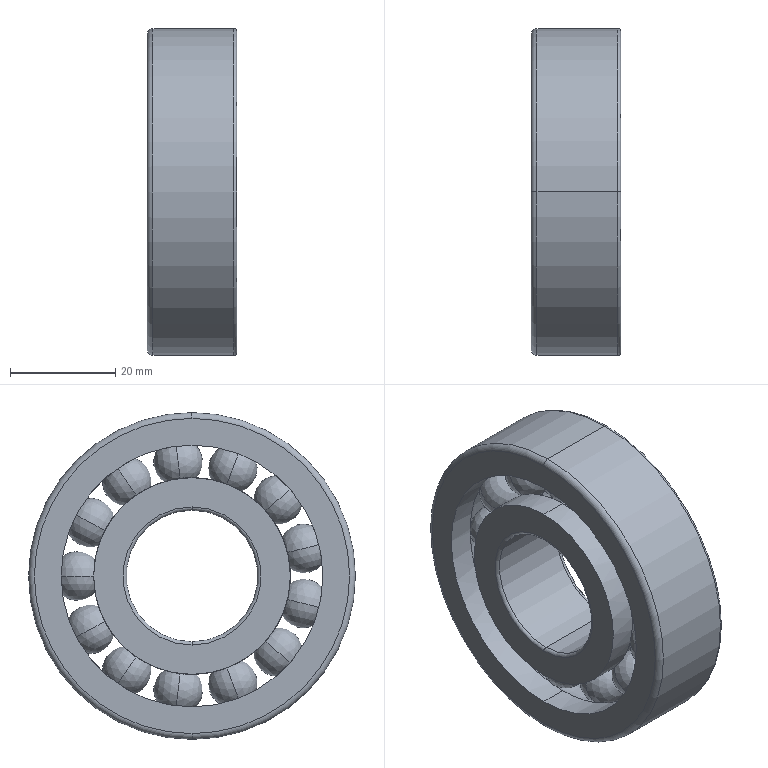Part | SolidWorks | features Revolution 3, Fillet 2, CirPattern 1 | 1 solid | 95 faces | box 17 x 62 x 62 mm | volume 31055 mm3 | torus 50 | sphere 26 | cylinder 14 | plane 5 | commonest cylinder face diameters 37.333 x4 25 x2 49.667 x2 51.157 x2 53.657 x2 62 x2